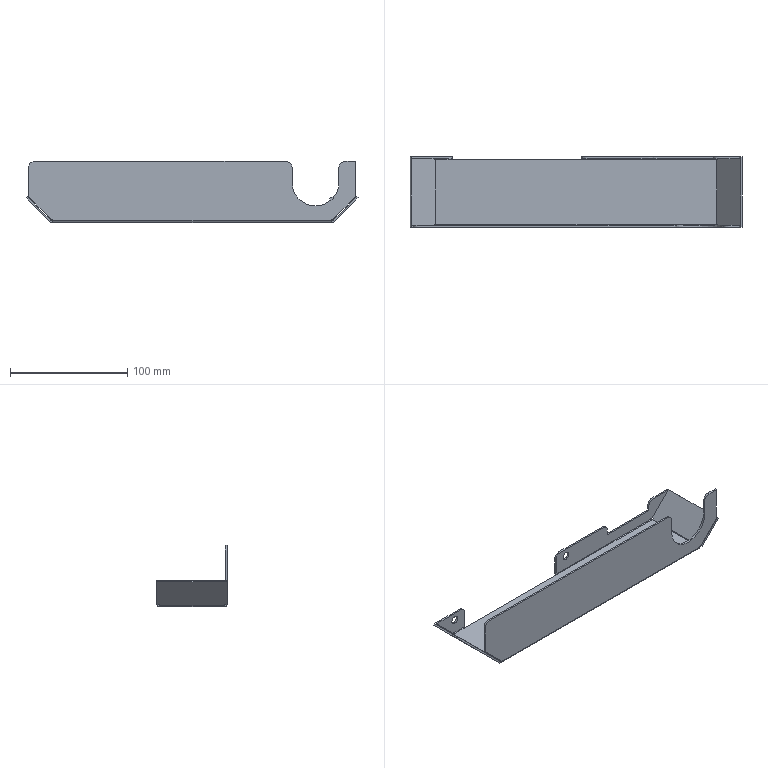Part | SolidWorks | features ICE 8, Fillet 3, Extrusion 1, FlatPattern 1, FlattenBends 1, ProcessBends 1, Rip 1, SheetMetal 1, Shell 1 | 1 solid | 95 faces | box 282.879 x 60 x 52 mm | volume 48298 mm3 | plane 73 | cylinder 22 | commonest cylinder face diameters 10 x7 1 x5 4 x5 7 x4 40 x1